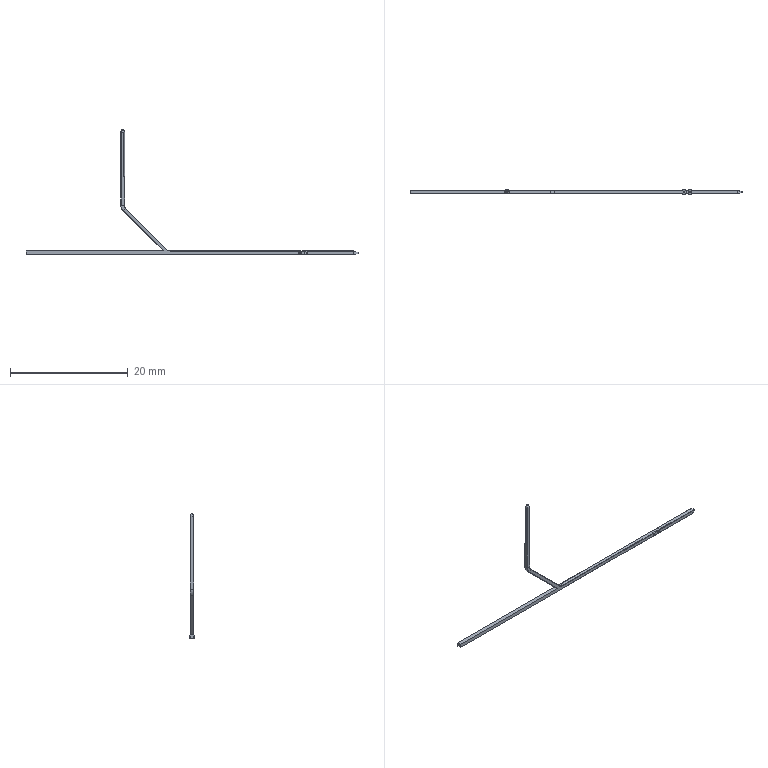Part | NX | features BREP 1 | 1 solid | 223 faces | box 56.43 x 0.8779 x 21.316 mm | volume 31.307 mm3 | cylinder 91 | plane 82 | torus 26 | sphere 20 | spline 4 | commonest cylinder face diameters 0.1 x32 0.09 x28 0.2 x12 2.01 x8 1 x4 2 x4